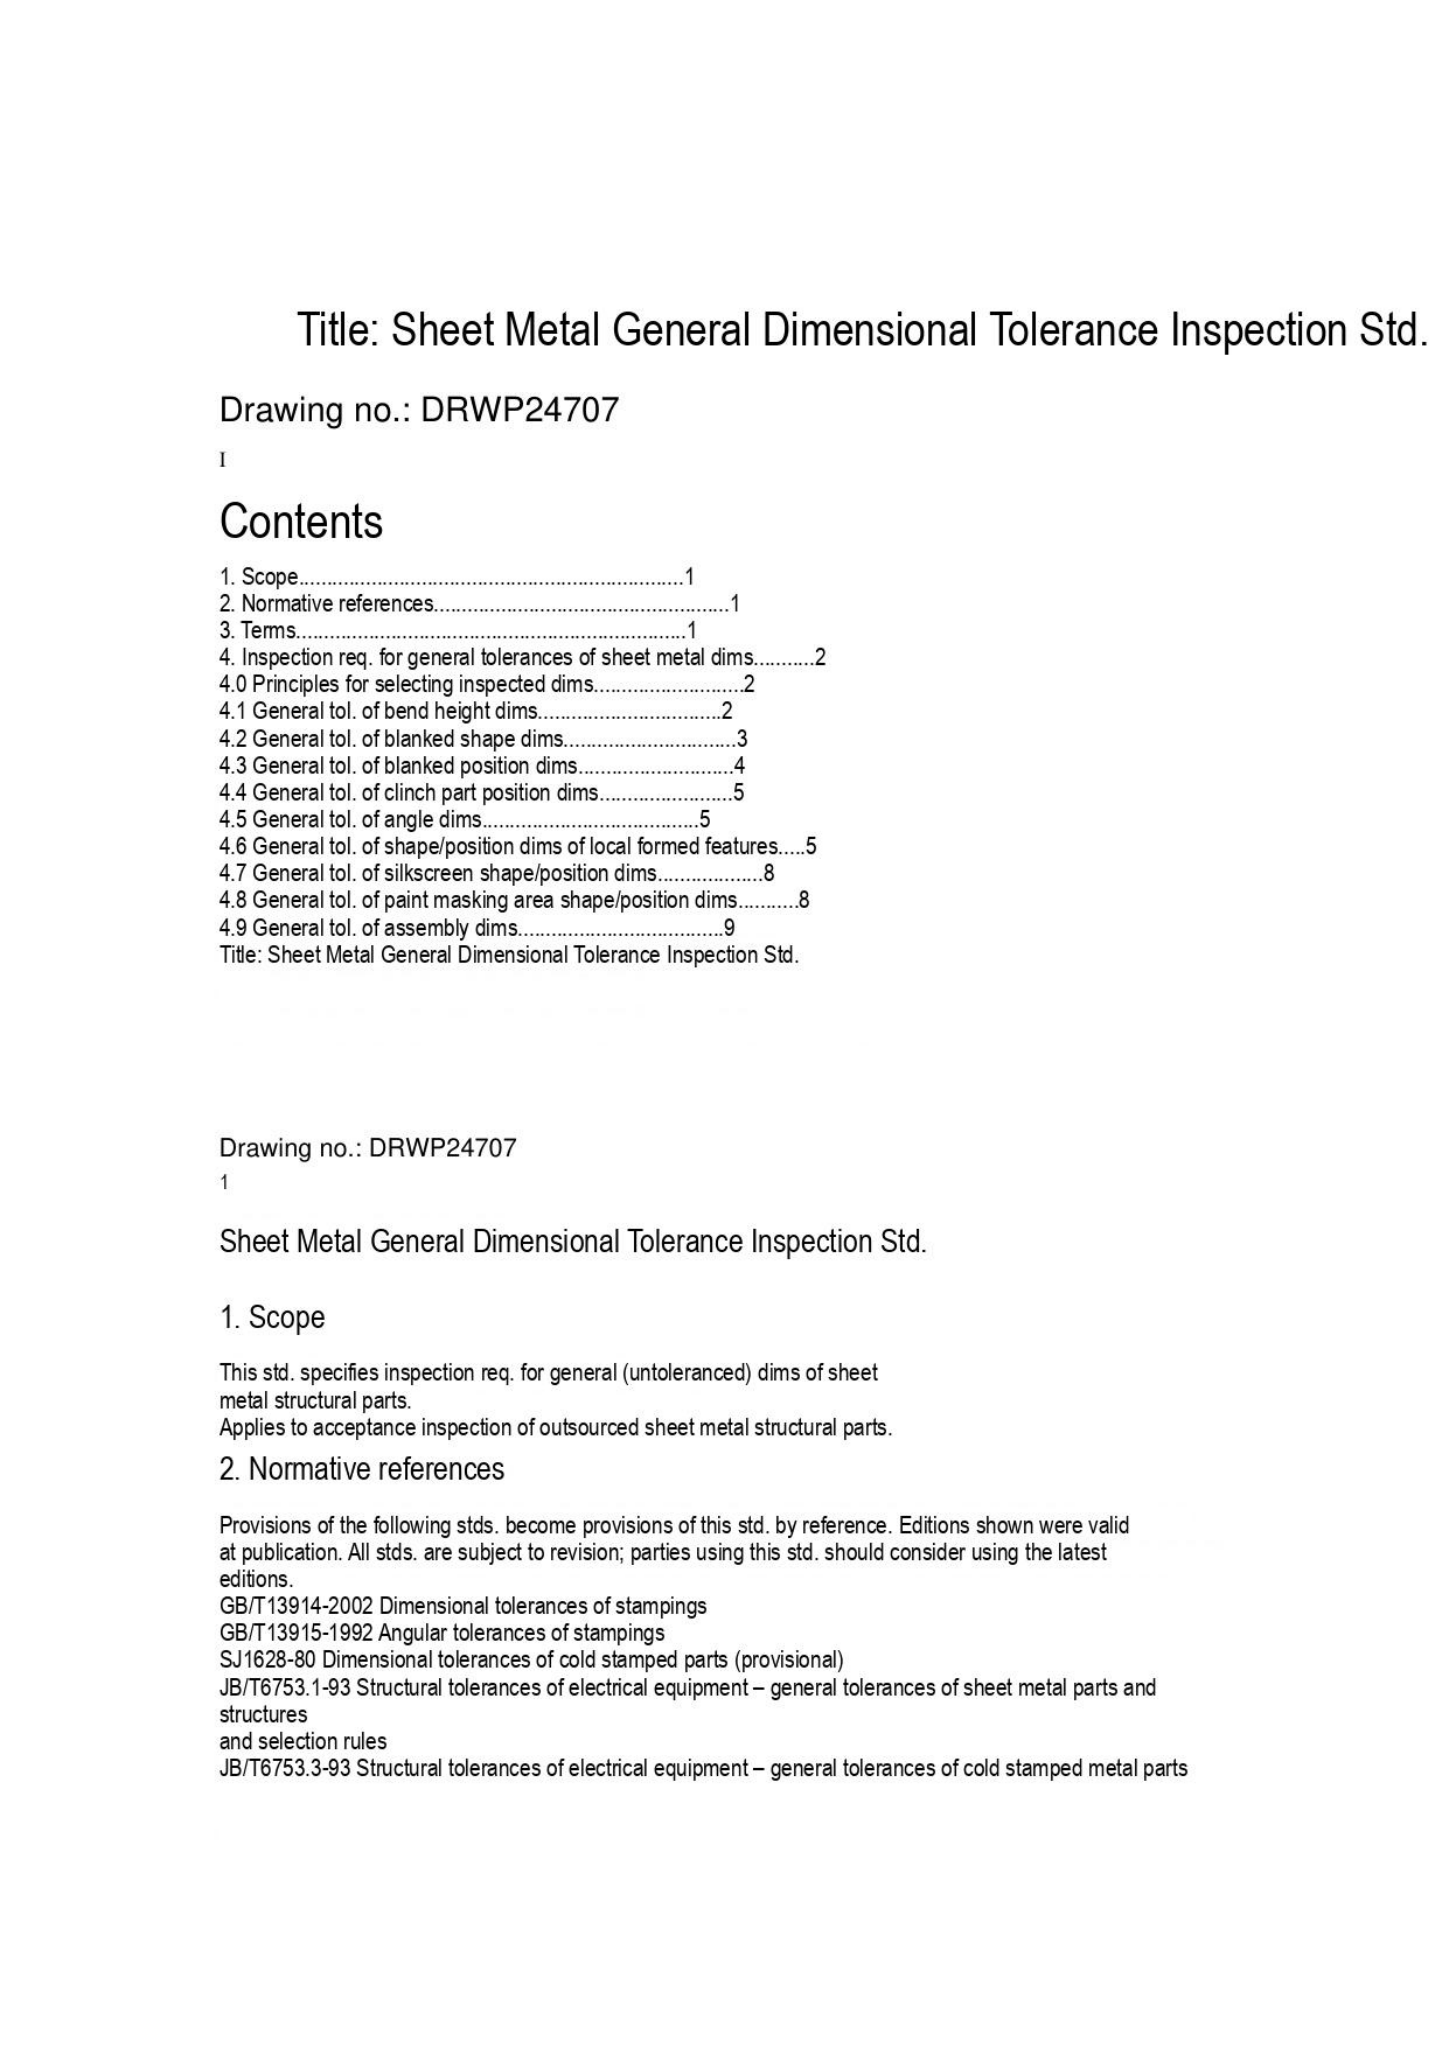Title: Sheet Metal General Dimensional Tolerance Inspection Std.

Drawing no.: DRWP24707

I

Contents

1. Scope.....................................................................1
2. Normative references.....................................................1
3. Terms.....................................................................1
4. Inspection req. for general tolerances of sheet metal dims...........2
4.0 Principles for selecting inspected dims...........................2
4.1 General tol. of bend height dims.................................2
4.2 General tol. of blanked shape dims...............................3
4.3 General tol. of blanked position dims............................4
4.4 General tol. of clinch part position dims........................5
4.5 General tol. of angle dims.......................................5
4.6 General tol. of shape/position dims of local formed features.....5
4.7 General tol. of silkscreen shape/position dims..................8
4.8 General tol. of paint masking area shape/position dims...........8
4.9 General tol. of assembly dims....................................9
Title: Sheet Metal General Dimensional Tolerance Inspection Std.

Drawing no.: DRWP24707
1

Sheet Metal General Dimensional Tolerance Inspection Std.

1. Scope

This std. specifies inspection req. for general (untoleranced) dims of sheet
metal structural parts.
Applies to acceptance inspection of outsourced sheet metal structural parts.

2. Normative references

Provisions of the following stds. become provisions of this std. by reference. Editions shown were valid
at publication. All stds. are subject to revision; parties using this std. should consider using the latest
editions.
GB/T13914-2002 Dimensional tolerances of stampings
GB/T13915-1992 Angular tolerances of stampings
SJ1628-80 Dimensional tolerances of cold stamped parts (provisional)
JB/T6753.1-93 Structural tolerances of electrical equipment – general tolerances of sheet metal parts and
structures
and selection rules
JB/T6753.3-93 Structural tolerances of electrical equipment – general tolerances of cold stamped metal parts
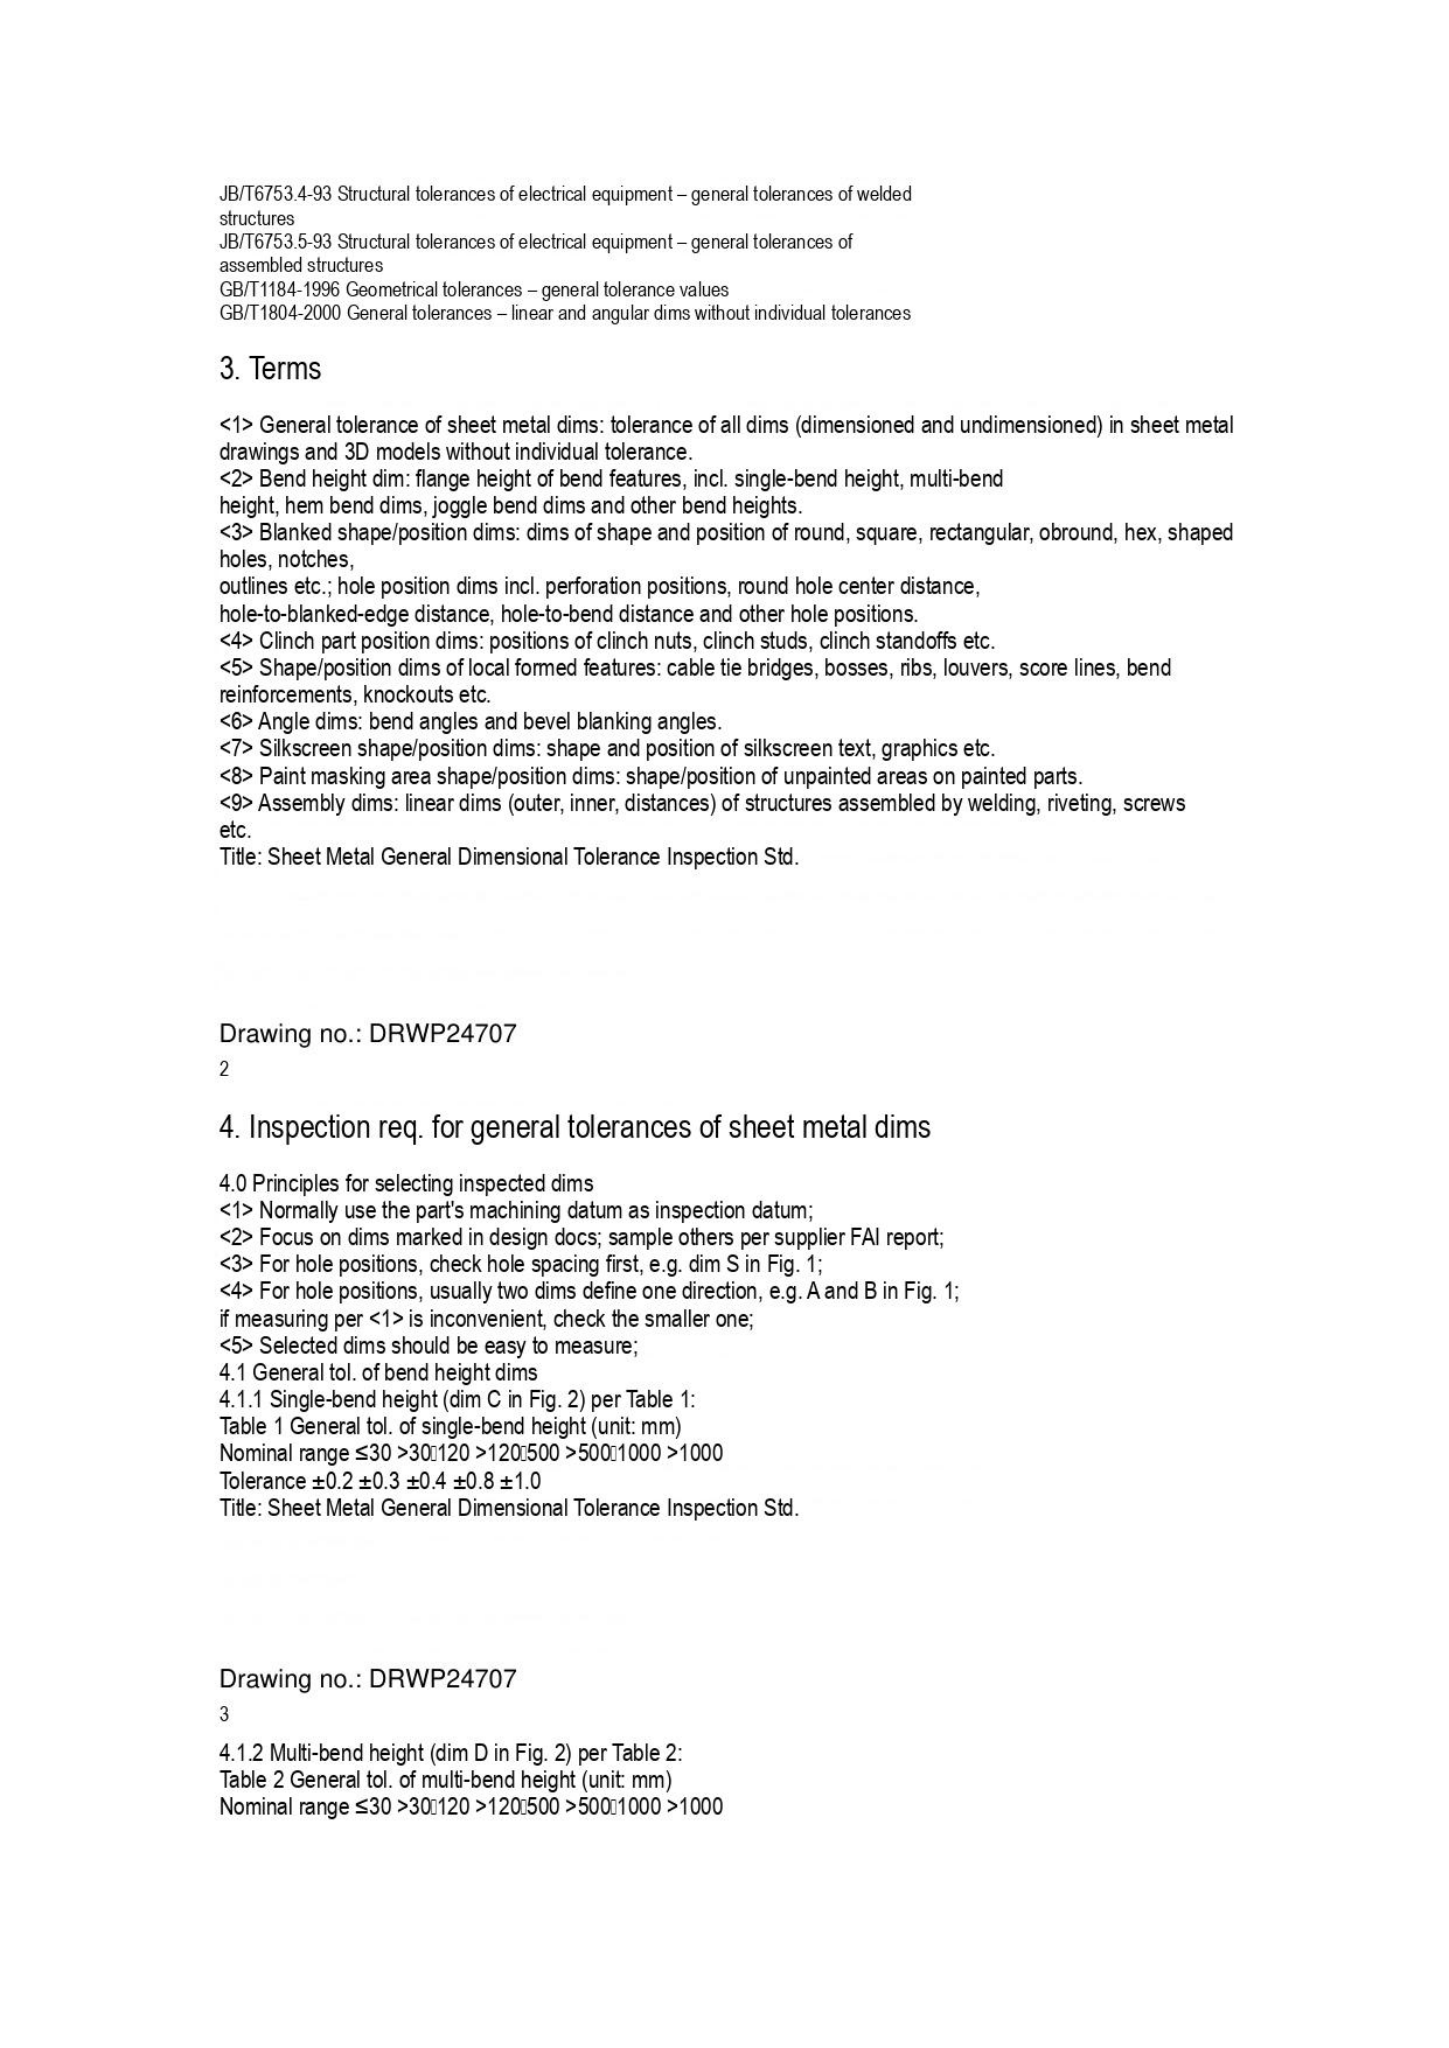JB/T6753.4-93 Structural tolerances of electrical equipment – general tolerances of welded structures
JB/T6753.5-93 Structural tolerances of electrical equipment – general tolerances of assembled structures
GB/T1184-1996 Geometrical tolerances – general tolerance values
GB/T1804-2000 General tolerances – linear and angular dims without individual tolerances

# 3. Terms

<1> General tolerance of sheet metal dims: tolerance of all dims (dimensioned and undimensioned) in sheet metal drawings and 3D models without individual tolerance.
<2> Bend height dim: flange height of bend features, incl. single-bend height, multi-bend height, hem bend dims, joggle bend dims and other bend heights.
<3> Blanked shape/position dims: dims of shape and position of round, square, rectangular, obround, hex, shaped holes, notches,
outlines etc.; hole position dims incl. perforation positions, round hole center distance,
hole-to-blanked-edge distance, hole-to-bend distance and other hole positions.
<4> Clinch part position dims: positions of clinch nuts, clinch studs, clinch standoffs etc.
<5> Shape/position dims of local formed features: cable tie bridges, bosses, ribs, louvers, score lines, bend reinforcements, knockouts etc.
<6> Angle dims: bend angles and bevel blanking angles.
<7> Silkscreen shape/position dims: shape and position of silkscreen text, graphics etc.
<8> Paint masking area shape/position dims: shape/position of unpainted areas on painted parts.
<9> Assembly dims: linear dims (outer, inner, distances) of structures assembled by welding, riveting, screws etc.
Title: Sheet Metal General Dimensional Tolerance Inspection Std.

Drawing no.: DRWP24707
2

# 4. Inspection req. for general tolerances of sheet metal dims

4.0 Principles for selecting inspected dims
<1> Normally use the part's machining datum as inspection datum;
<2> Focus on dims marked in design docs; sample others per supplier FAI report;
<3> For hole positions, check hole spacing first, e.g. dim S in Fig. 1;
<4> For hole positions, usually two dims define one direction, e.g. A and B in Fig. 1;
if measuring per <1> is inconvenient, check the smaller one;
<5> Selected dims should be easy to measure;
4.1 General tol. of bend height dims
4.1.1 Single-bend height (dim C in Fig. 2) per Table 1:
Table 1 General tol. of single-bend height (unit: mm)

| Nominal range | ≤30 | >30□120 | >120□500 | >500□1000 | >1000 |
|---|---|---|---|---|---|
| Tolerance | ±0.2 | ±0.3 | ±0.4 | ±0.8 | ±1.0 |

Title: Sheet Metal General Dimensional Tolerance Inspection Std.

Drawing no.: DRWP24707
3

4.1.2 Multi-bend height (dim D in Fig. 2) per Table 2:
Table 2 General tol. of multi-bend height (unit: mm)

| Nominal range | ≤30 | >30□120 | >120□500 | >500□1000 | >1000 |
|---|---|---|---|---|---|
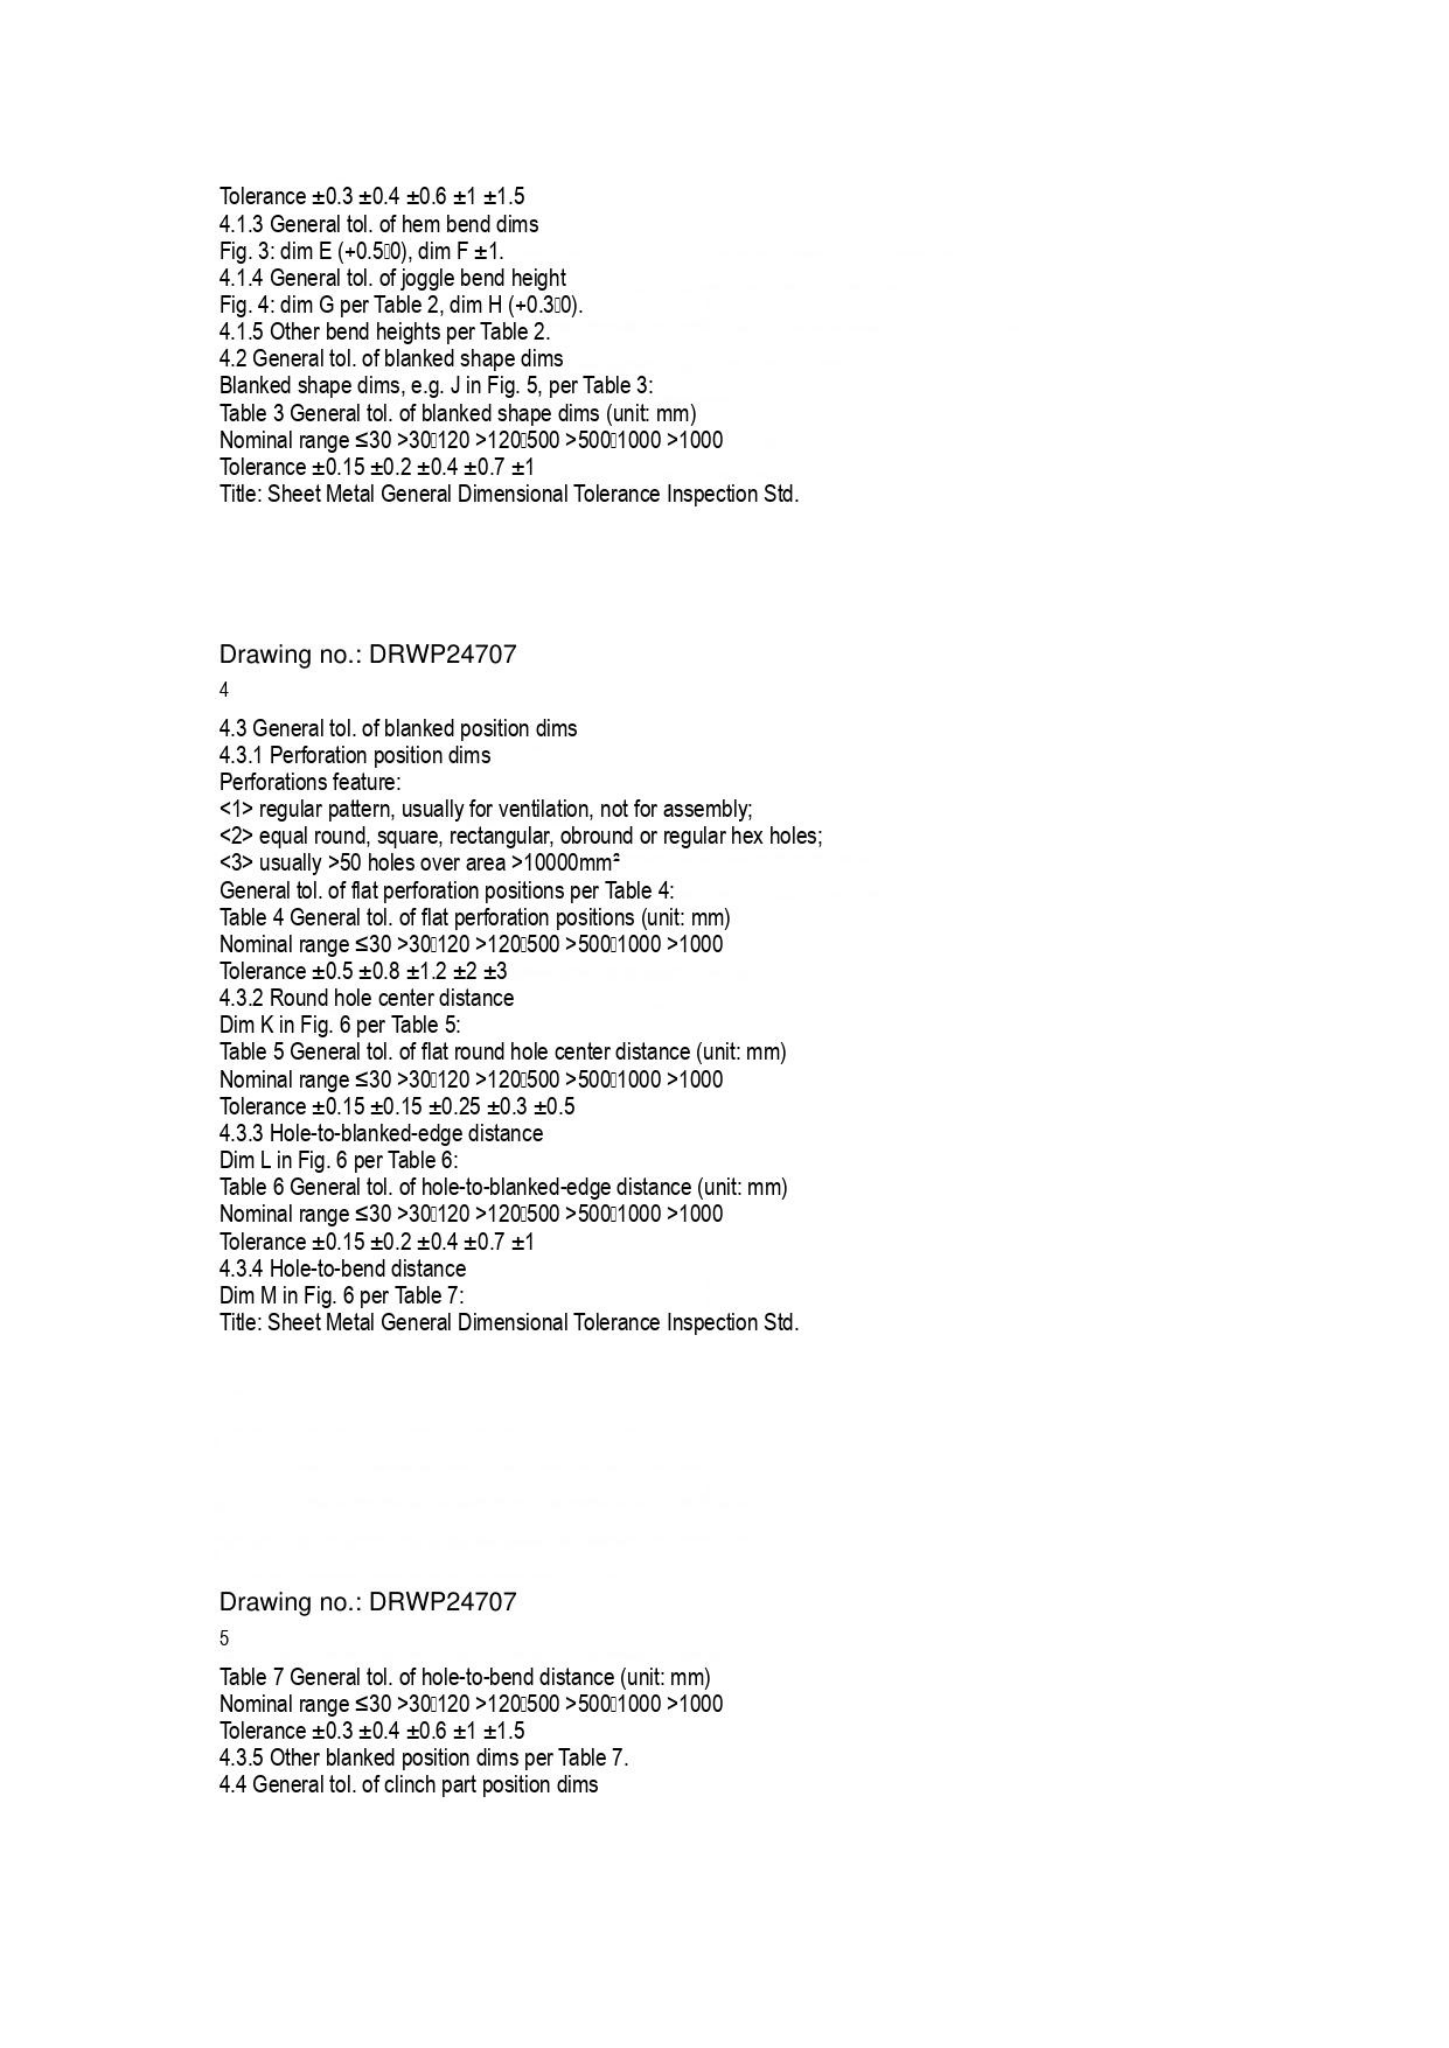Tolerance ±0.3 ±0.4 ±0.6 ±1 ±1.5
4.1.3 General tol. of hem bend dims
Fig. 3: dim E (+0.5□0), dim F ±1.
4.1.4 General tol. of joggle bend height
Fig. 4: dim G per Table 2, dim H (+0.3□0).
4.1.5 Other bend heights per Table 2.
4.2 General tol. of blanked shape dims
Blanked shape dims, e.g. J in Fig. 5, per Table 3:
Table 3 General tol. of blanked shape dims (unit: mm)

| Nominal range | ≤30 | >30□120 | >120□500 | >500□1000 | >1000 |
|---|---|---|---|---|---|
| Tolerance | ±0.15 | ±0.2 | ±0.4 | ±0.7 | ±1 |

Title: Sheet Metal General Dimensional Tolerance Inspection Std.

Drawing no.: DRWP24707
4

4.3 General tol. of blanked position dims
4.3.1 Perforation position dims
Perforations feature:
<1> regular pattern, usually for ventilation, not for assembly;
<2> equal round, square, rectangular, obround or regular hex holes;
<3> usually >50 holes over area >10000mm²
General tol. of flat perforation positions per Table 4:
Table 4 General tol. of flat perforation positions (unit: mm)

| Nominal range | ≤30 | >30□120 | >120□500 | >500□1000 | >1000 |
|---|---|---|---|---|---|
| Tolerance | ±0.5 | ±0.8 | ±1.2 | ±2 | ±3 |

4.3.2 Round hole center distance
Dim K in Fig. 6 per Table 5:
Table 5 General tol. of flat round hole center distance (unit: mm)

| Nominal range | ≤30 | >30□120 | >120□500 | >500□1000 | >1000 |
|---|---|---|---|---|---|
| Tolerance | ±0.15 | ±0.15 | ±0.25 | ±0.3 | ±0.5 |

4.3.3 Hole-to-blanked-edge distance
Dim L in Fig. 6 per Table 6:
Table 6 General tol. of hole-to-blanked-edge distance (unit: mm)

| Nominal range | ≤30 | >30□120 | >120□500 | >500□1000 | >1000 |
|---|---|---|---|---|---|
| Tolerance | ±0.15 | ±0.2 | ±0.4 | ±0.7 | ±1 |

4.3.4 Hole-to-bend distance
Dim M in Fig. 6 per Table 7:
Title: Sheet Metal General Dimensional Tolerance Inspection Std.

Drawing no.: DRWP24707
5

Table 7 General tol. of hole-to-bend distance (unit: mm)

| Nominal range | ≤30 | >30□120 | >120□500 | >500□1000 | >1000 |
|---|---|---|---|---|---|
| Tolerance | ±0.3 | ±0.4 | ±0.6 | ±1 | ±1.5 |

4.3.5 Other blanked position dims per Table 7.
4.4 General tol. of clinch part position dims
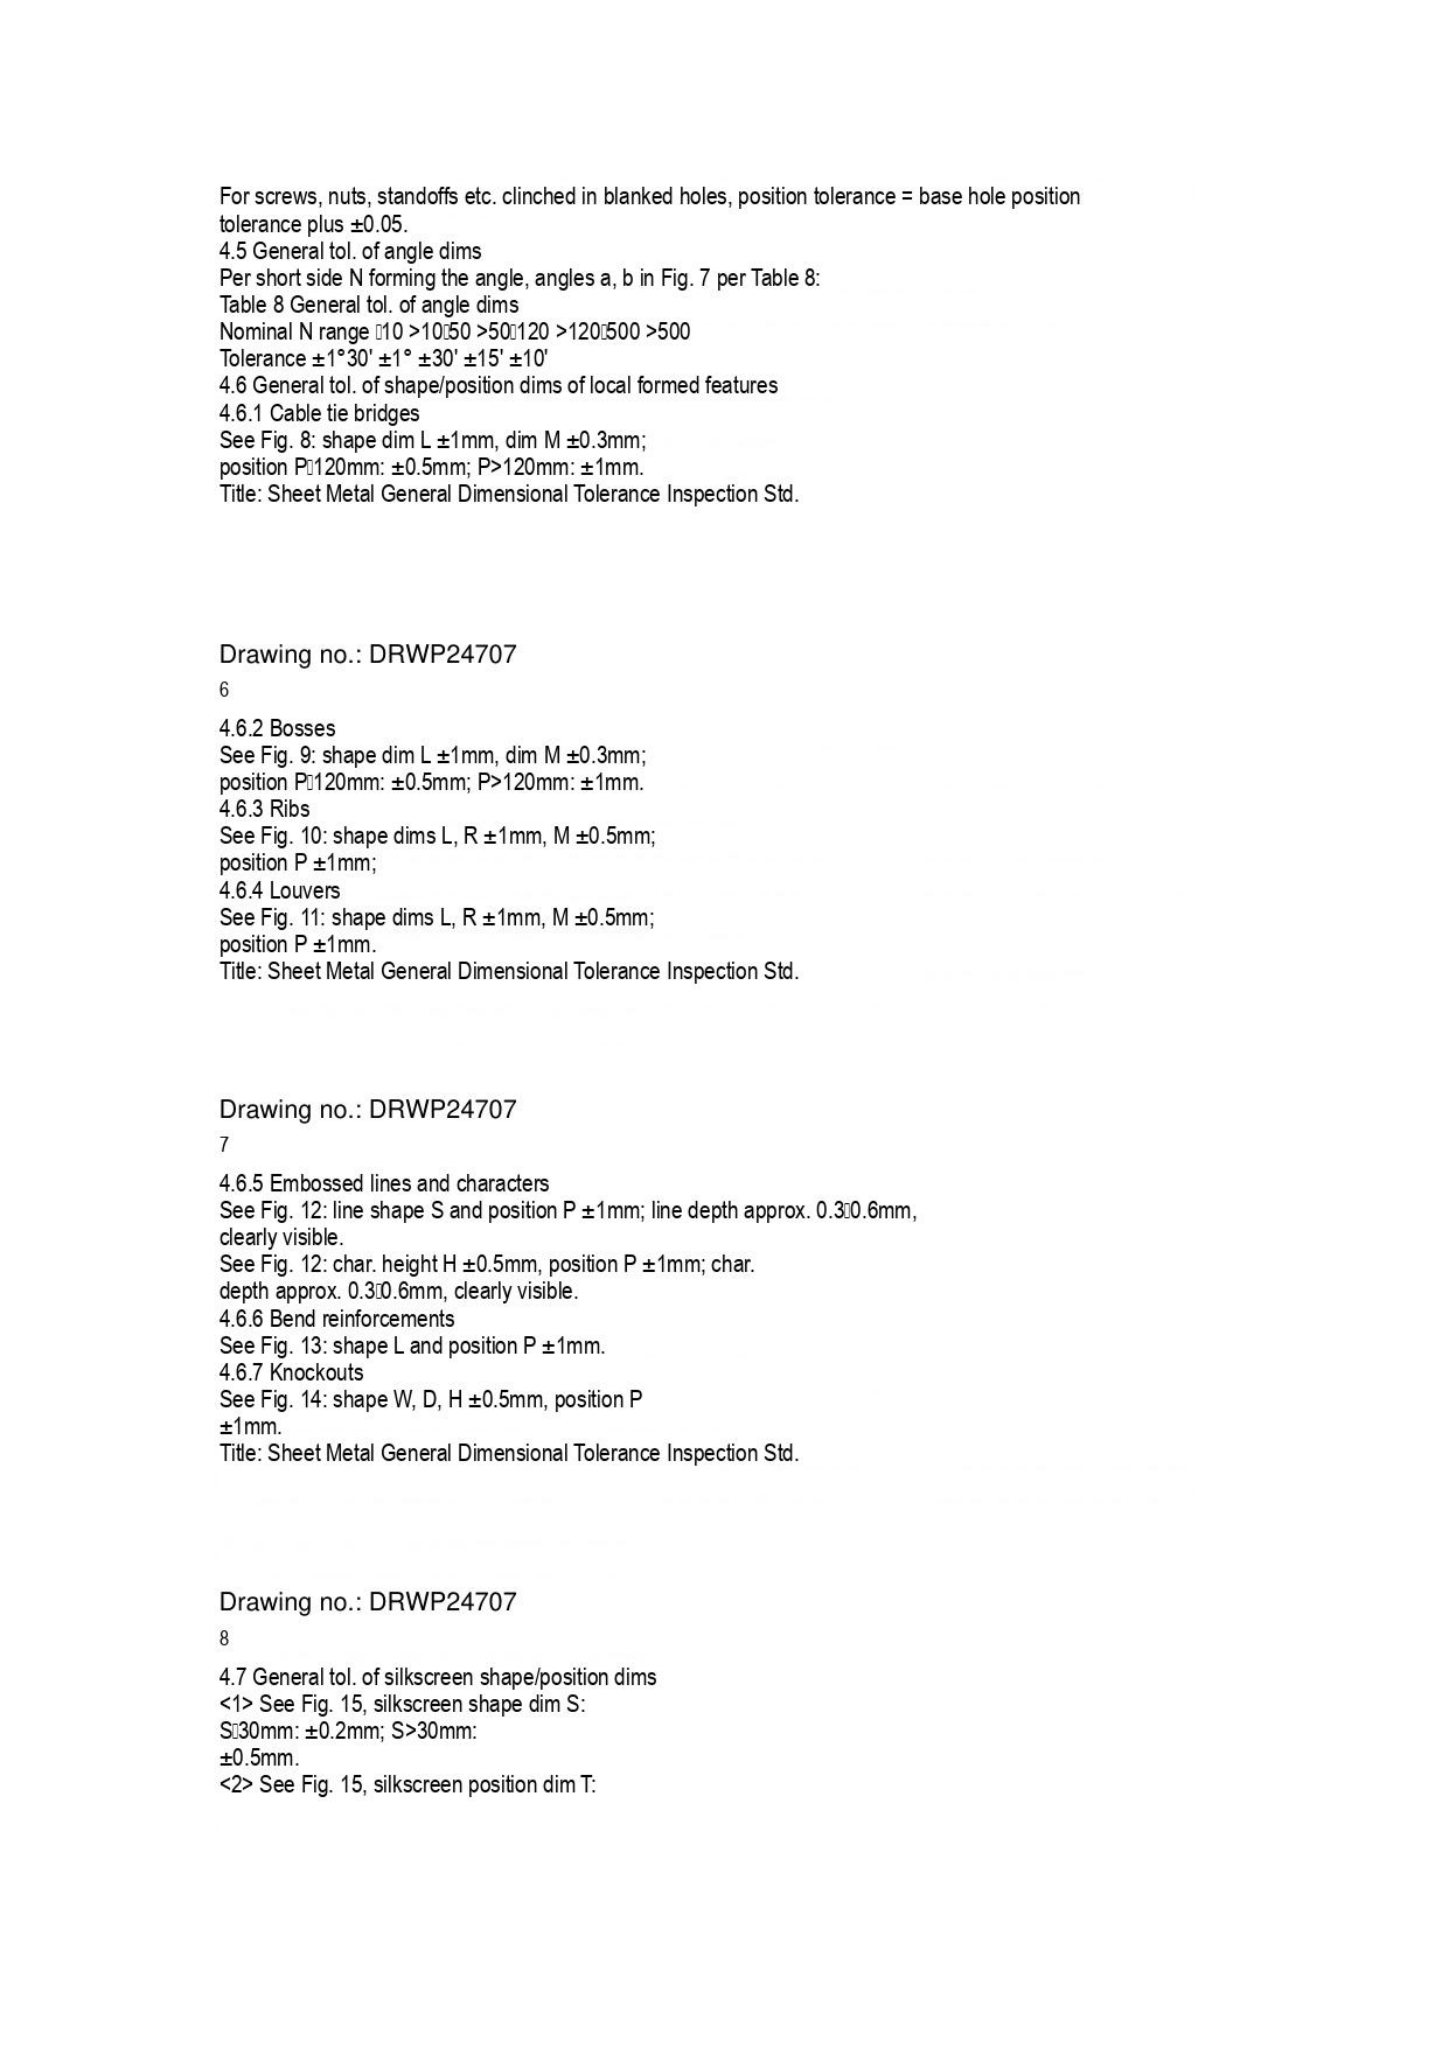For screws, nuts, standoffs etc. clinched in blanked holes, position tolerance = base hole position tolerance plus ±0.05.
4.5 General tol. of angle dims
Per short side N forming the angle, angles a, b in Fig. 7 per Table 8:
Table 8 General tol. of angle dims
Nominal N range □10 >10□50 >50□120 >120□500 >500
Tolerance ±1°30' ±1° ±30' ±15' ±10'
4.6 General tol. of shape/position dims of local formed features
4.6.1 Cable tie bridges
See Fig. 8: shape dim L ±1mm, dim M ±0.3mm;
position P□120mm: ±0.5mm; P>120mm: ±1mm.
Title: Sheet Metal General Dimensional Tolerance Inspection Std.

Drawing no.: DRWP24707
6

4.6.2 Bosses
See Fig. 9: shape dim L ±1mm, dim M ±0.3mm;
position P□120mm: ±0.5mm; P>120mm: ±1mm.
4.6.3 Ribs
See Fig. 10: shape dims L, R ±1mm, M ±0.5mm;
position P ±1mm;
4.6.4 Louvers
See Fig. 11: shape dims L, R ±1mm, M ±0.5mm;
position P ±1mm.
Title: Sheet Metal General Dimensional Tolerance Inspection Std.

Drawing no.: DRWP24707
7

4.6.5 Embossed lines and characters
See Fig. 12: line shape S and position P ±1mm; line depth approx. 0.3□0.6mm, clearly visible.
See Fig. 12: char. height H ±0.5mm, position P ±1mm; char. depth approx. 0.3□0.6mm, clearly visible.
4.6.6 Bend reinforcements
See Fig. 13: shape L and position P ±1mm.
4.6.7 Knockouts
See Fig. 14: shape W, D, H ±0.5mm, position P ±1mm.
Title: Sheet Metal General Dimensional Tolerance Inspection Std.

Drawing no.: DRWP24707
8

4.7 General tol. of silkscreen shape/position dims
<1> See Fig. 15, silkscreen shape dim S:
S□30mm: ±0.2mm; S>30mm:
±0.5mm.
<2> See Fig. 15, silkscreen position dim T:
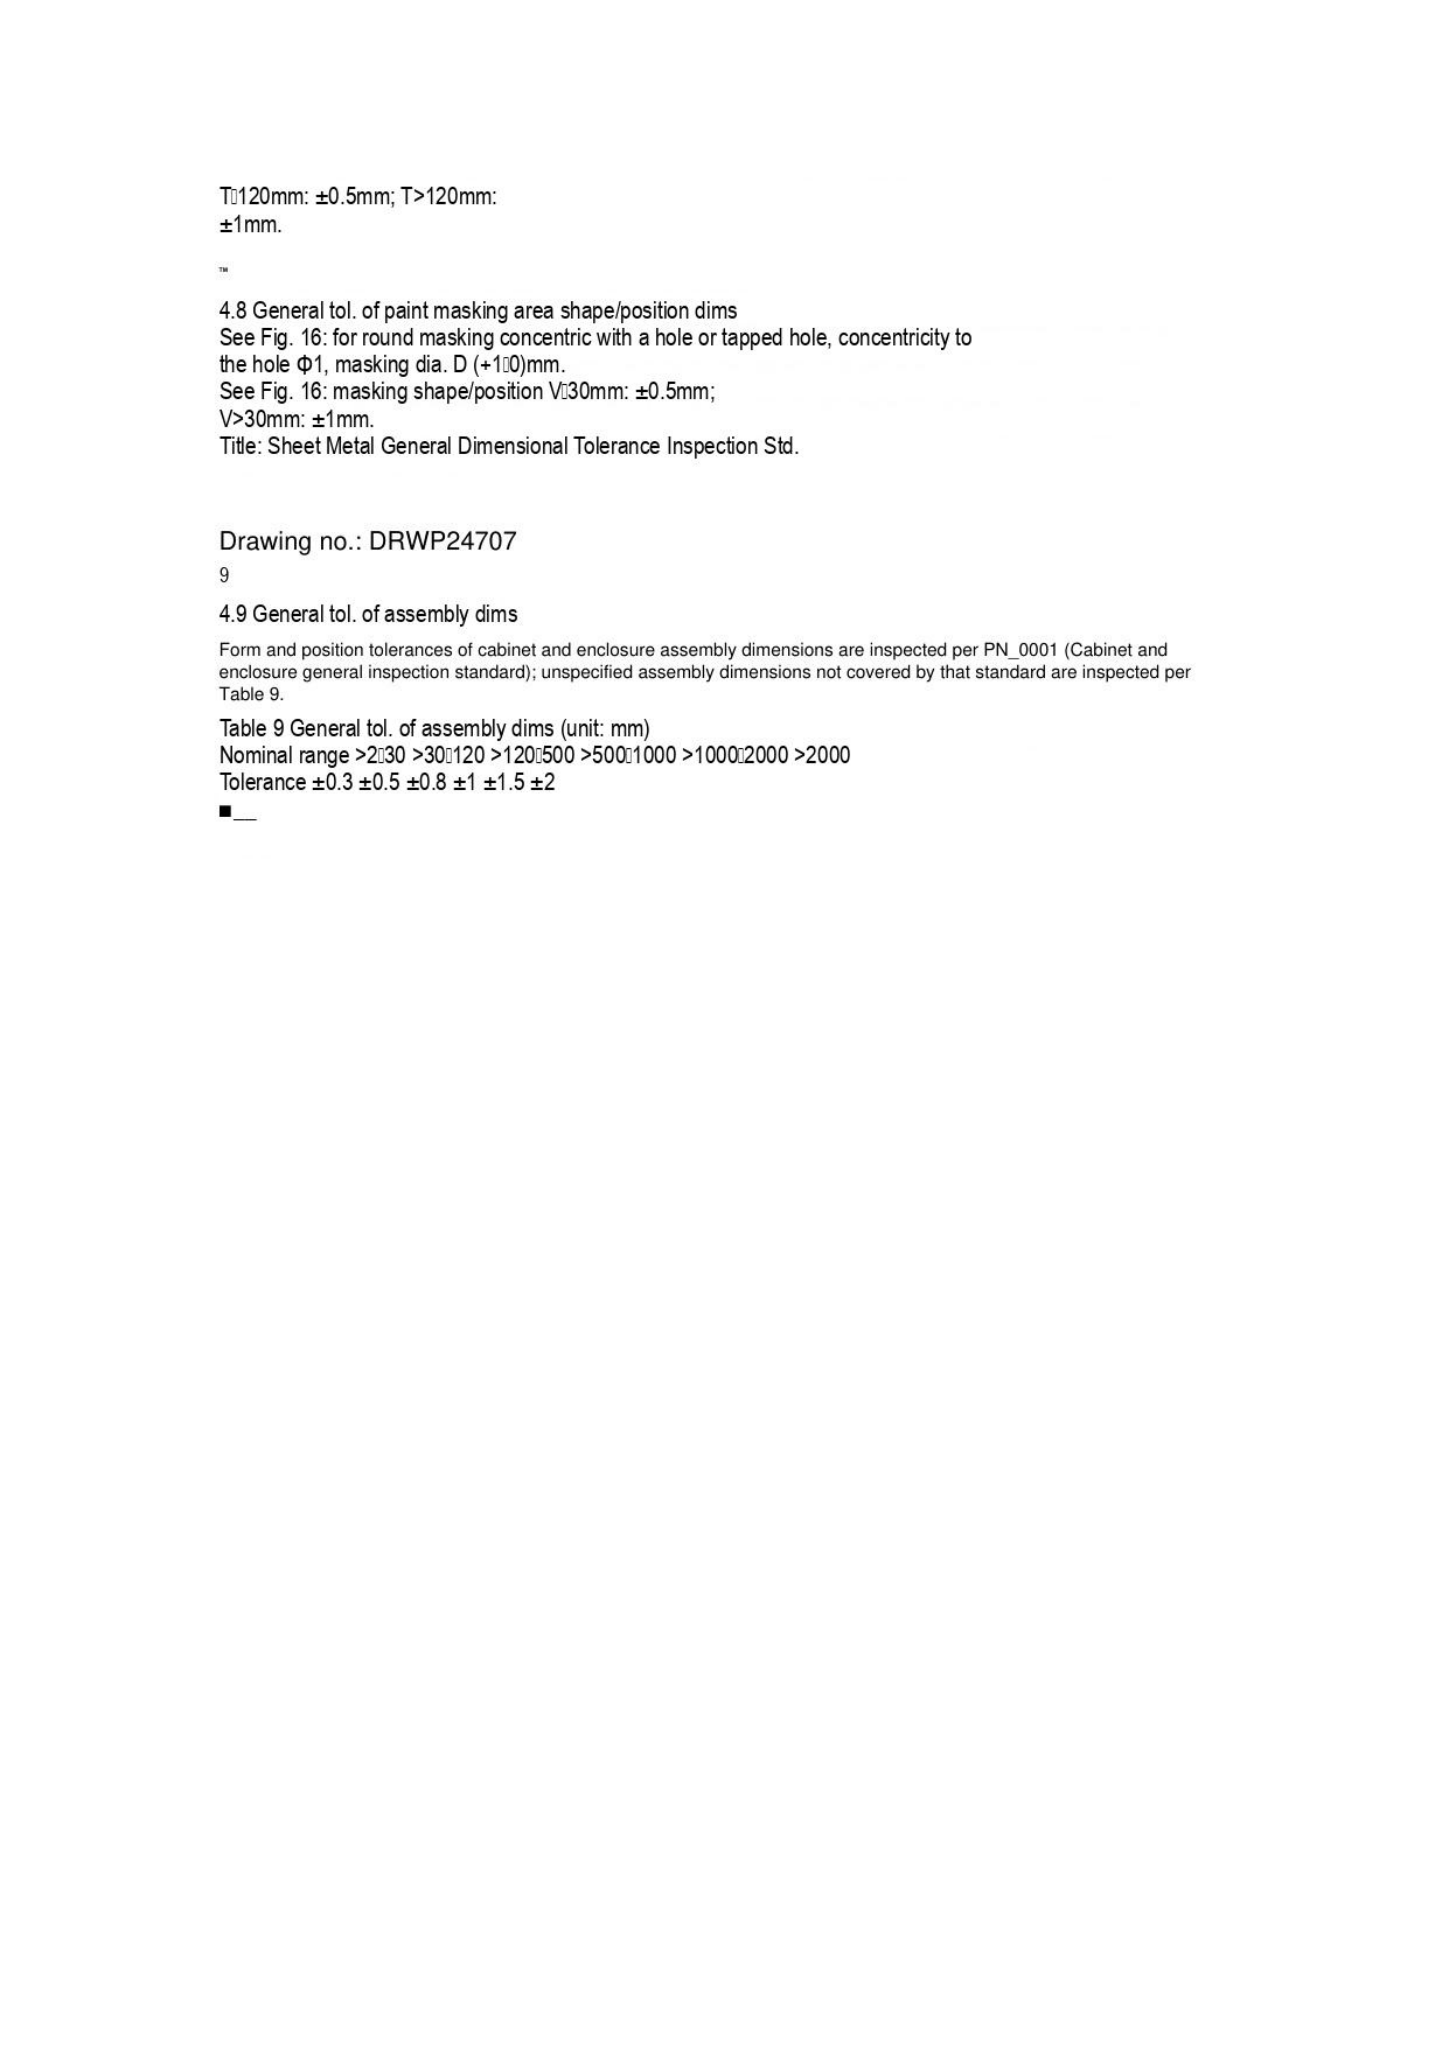T120mm: ±0.5mm; T>120mm:
±1mm.

™

4.8 General tol. of paint masking area shape/position dims
See Fig. 16: for round masking concentric with a hole or tapped hole, concentricity to the hole Φ1, masking dia. D (+10)mm.
See Fig. 16: masking shape/position V30mm: ±0.5mm;
V>30mm: ±1mm.
Title: Sheet Metal General Dimensional Tolerance Inspection Std.

Drawing no.: DRWP24707
9

4.9 General tol. of assembly dims

Form and position tolerances of cabinet and enclosure assembly dimensions are inspected per PN_0001 (Cabinet and enclosure general inspection standard); unspecified assembly dimensions not covered by that standard are inspected per Table 9.

Table 9 General tol. of assembly dims (unit: mm)

| Nominal range | >230 | >30120 | >120500 | >5001000 | >10002000 | >2000 |
|---|---|---|---|---|---|---|
| Tolerance | ±0.3 | ±0.5 | ±0.8 | ±1 | ±1.5 | ±2 |

■__